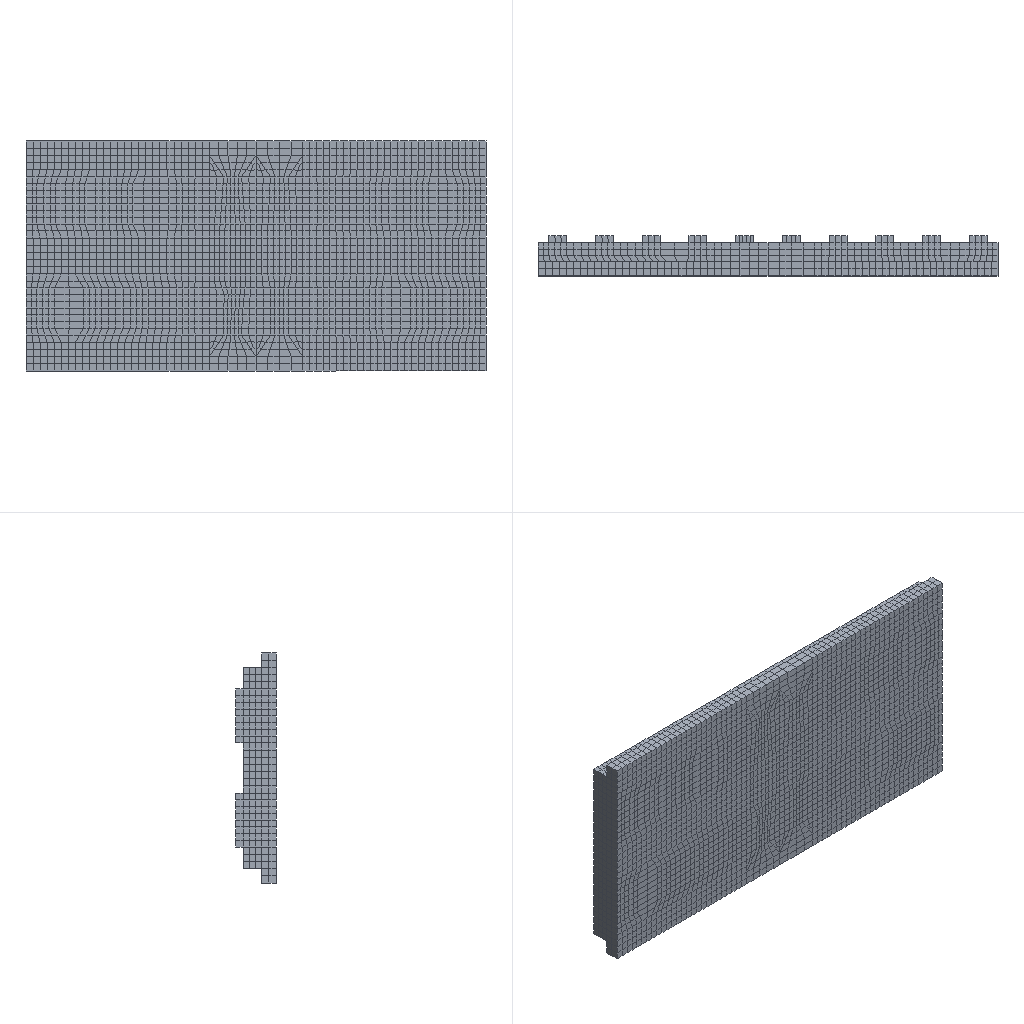Simulation study | abaqus
Set-up summary:
category,name,step,type,value,unit,region
solver,abaqus
solver,version,,,Abaqus/Explicit 2020
units,not stated in the deck,,not stated
analysis,deck,,transient,transient
load_step,Step-1,Step-1,transient,nlgeom=True
contact,interactions,,,general=0 pairs=0 ties=0
load_step,requested,,,1
mesh,nodes,,,15496
mesh,elements,,,12702
element_type,T3D2,,truss,1496
element_type,C3D8R,,solid,11134
element_type,COH3D8,,cohesive,72
load,load commands in deck,,count,1
bc,support commands in deck,,count,1
material,CONCRETE-COPY,,in results
material,CRACK,,in results
material,STEEL,,in results
check,setup vs results,,match,"per instance, exact: element labels, types and connectivity; labels of the nodes the elements use; coordinates not compared"
Abaqus input file, long lists of numbers shortened:
*Heading
** Job name: Job-2 Model name: Model-1
** Generated by: Abaqus/CAE 2020
*Preprint, echo=NO, model=NO, history=NO, contact=NO
**
** PARTS
**
*Part, name=concrete-final
*Node
      1,   4431.458,   309.396,        2750.
      2,   4431.458,   309.396,        3000.
** (14444 more lines like these left out)
*Element, type=C3D8R
 1,     4,   270,  2617,   277, 14216, 14215,  9263,  2648
 2,   270,   269,  2618,  2617, 14215, 14217,  9264,  9263
** (11132 more lines like these left out)
*Element, type=COH3D8
11135,   287,  2653,   270,     4, 14216, 14215,   270,     4
11136,  2653,  2654,   269,   270, 14215, 14217,   269,   270
** (70 more lines like these left out)
*Nset, nset=Set-17
     1,     2,     4,     5,     6,     7,     9,    10,    11,    12,    13,    14,    15,    16,    17,    18
    19,    20,    21,    22,    23,    24,    25,    26,    27,    28,    29,    30,    31,    32,    33,    34
** (851 more lines like these left out)
*Elset, elset=Set-17
   112,   113,   114,   115,   116,   117,   118,   119,   120,   121,   122,   123,   124,   125,   126,   127
   128,   129,   130,   131,   132,   133,   134,   135,   136,   137,   138,   139,   140,   141,   142,   143
** (660 more lines like these left out)
*Nset, nset=Set-22, generate
     1,  14286,      1
*Elset, elset=Set-22, generate
     1,  11134,      1
*Elset, elset=CohesiveSeam-2-Elements, generate
 11135,  11206,      1
*Nset, nset=CohesiveSeam-2-TopNodes
     1,     2,     3,     4,     6,     7,    11,    12,    13,    14,    15,    31,    32,    34,    49,    50
    51,    53,    54,    55,    56,    57,   269,   270,   275,   276,   281,   282,   283,   284,   309,   310
** (6 more lines like these left out)
*Nset, nset=CohesiveSeam-2-BottomNodes
    1,    2,    3,    4,    5,    6,    7,    8,   11,   12,   13,   14,   15,   16,   31,   32
   34,   35,   49,   50,   51,   52,   53,   54,   55,   56,   57,   58,  269,  270,  275,  276
** (6 more lines like these left out)
*Nset, nset=CohesiveSeam-2-MidNodes
   1,   2,   3,   4,   6,   7,  11,  12,  13,  14,  15,  31,  32,  34,  49,  50
  51,  53,  54,  55,  56,  57, 269, 270, 275, 276, 281, 282, 283, 284, 309, 310
** (2 more lines like these left out)
*Elset, elset=__PickedSurf72_S1, internal
 11135, 11136, 11137, 11138, 11139, 11140, 11141, 11142, 11143, 11153, 11154, 11155, 11156, 11157, 11158, 11159
 11160, 11161, 11189, 11190, 11191, 11192, 11193, 11194, 11195, 11196, 11197
*Elset, elset=__PickedSurf72_S2, internal
 11144, 11145, 11146, 11147, 11148, 11149, 11150, 11151, 11152, 11162, 11163, 11164, 11165, 11166, 11167, 11168
 11169, 11170, 11171, 11172, 11173, 11174, 11175, 11176, 11177, 11178, 11179, 11180, 11181, 11182, 11183, 11184
** (1 more lines like these left out)
*Surface, type=ELEMENT, name=_PickedSurf72, internal
__PickedSurf72_S1, S1
__PickedSurf72_S2, S2
*Elset, elset=_CohesiveSeam-2-TopSurf_S2, internal, generate
 11135,  11206,      1
*Surface, type=ELEMENT, name=CohesiveSeam-2-TopSurf
_CohesiveSeam-2-TopSurf_S2, S2
*Elset, elset=_CohesiveSeam-2-BottomSurf_S1, internal, generate
 11135,  11206,      1
*Surface, type=ELEMENT, name=CohesiveSeam-2-BottomSurf
_CohesiveSeam-2-BottomSurf_S1, S1
** Section: Section-1-SET-1
*Solid Section, elset=Set-22, material=CONCRETE-Copy
,
** Section: Section-coh
*Cohesive Section, elset=CohesiveSeam-2-Elements, controls=EC-1, material=crack, response=TRACTION SEPARATION, thickness=SPECIFIED
0.1,
*End Part
**
*Part, name="steel bar"
*Node
      1,       -1800.,        -350.,        2700.
      2,       -1400.,        -350.,        2700.
** (1048 more lines like these left out)
*Element, type=T3D2
   1,    1,  523
   2,  523,    2
** (1494 more lines like these left out)
*Nset, nset=SET-1, generate
    1,  1050,     1
*Elset, elset=SET-1, generate
    1,  1496,     1
*Nset, nset="'Set-300'", generate
    1,  1050,     1
*Nset, nset=Set-300
   1,  29,  37, 242, 266, 274, 350, 429
** Section: Section-2-SET-1
*Solid Section, elset=SET-1, material=STEEL
201.1,
*End Part
**
**
** ASSEMBLY
**
*Assembly, name=Assembly
**
*Instance, name="steel bar-1", part="steel bar"
*End Instance
**
*Instance, name=concrete-final-1, part=concrete-final
      -1850.,  -709.396,  4731.457
      -1850.,  -709.396,  4731.457,       -1850., -708.396,  4731.457, 90.
*End Instance
**
*Node
      1,        1025.,         -40.,        2125.
      2,        1675.,         -40.,        2125.
** (5 more lines like these left out)
*Nset, nset=M_SET-1
 1,
*Nset, nset=M_SET-2
 2,
*Nset, nset=M_SET-3
 4,
*Nset, nset=M_SET-4
 3,
*Nset, nset=M_SET-12
 6,
*Nset, nset=M_SET-13
 7,
*Nset, nset=M_SET-16
 5,
*Nset, nset=SET-10, generate
 1,  4,  1
*Nset, nset=SET-11
 5,
*Nset, nset=SET-14
 7,
*Nset, nset=SET-15
 6,
*Nset, nset=SET-17
 5,
*Nset, nset=Set-41, instance=concrete-final-1
   19,   20,   21,   22,   37,   38,   39,   40,   61,   62,   63,   64,   80,   81,   82,   83
   84,   86,   87,  112,  113,  114,  115,  116,  117,  141,  142,  143,  153,  154,  155,  156
** (22 more lines like these left out)
*Elset, elset=Set-41, instance=concrete-final-1
   346,   347,   348,   349,   350,   351,   352,   353,   354,   604,   605,   606,   607,   608,   609,   610
   611,   612,   934,   935,   936,   937,   938,   939,   940,   941,   942,  1263,  1264,  1265,  1266,  1267
** (18 more lines like these left out)
*Nset, nset=Set-42, generate
 1,  4,  1
*Nset, nset=WIRE-1-SET-2, instance="steel bar-1", generate
    1,  1050,     1
*Nset, nset=m_Set-35
 1,
*Nset, nset=m_Set-36
 2,
*Nset, nset=m_Set-37
 3,
*Nset, nset=m_Set-38
 4,
*Elset, elset=m_Set-39, instance="steel bar-1", generate
    1,  1496,     1
*Elset, elset=m_Set-42, instance="steel bar-1", generate
    1,  1496,     1
*Nset, nset=s_Set-39, instance=concrete-final-1
     1,     2,     4,     5,     6,     7,     9,    10,    11,    12,    13,    14,    15,    16,    17,    18
    19,    20,    21,    22,    23,    24,    25,    26,    27,    28,    29,    30,    31,    32,    33,    34
** (851 more lines like these left out)
*Elset, elset=s_Set-39, instance=concrete-final-1
   112,   113,   114,   115,   116,   117,   118,   119,   120,   121,   122,   123,   124,   125,   126,   127
   128,   129,   130,   131,   132,   133,   134,   135,   136,   137,   138,   139,   140,   141,   142,   143
** (660 more lines like these left out)
*Nset, nset=s_Set-42, instance=concrete-final-1, generate
     1,  14286,      1
*Elset, elset=s_Set-42, instance=concrete-final-1, generate
     1,  11134,      1
*Elset, elset=_s_Surf-9_S5, internal, instance=concrete-final-1, generate
 8271,  8310,     1
*Surface, type=ELEMENT, name=s_Surf-9
_s_Surf-9_S5, S5
*Elset, elset=_s_Surf-10_S5, internal, instance=concrete-final-1, generate
 5079,  5110,     1
*Surface, type=ELEMENT, name=s_Surf-10
_s_Surf-10_S5, S5
*Elset, elset=_s_Surf-11_S5, internal, instance=concrete-final-1, generate
 5207,  5238,     1
*Surface, type=ELEMENT, name=s_Surf-11
_s_Surf-11_S5, S5
*Elset, elset=_s_Surf-12_S5, internal, instance=concrete-final-1, generate
 6695,  6734,     1
*Surface, type=ELEMENT, name=s_Surf-12
_s_Surf-12_S5, S5
** Constraint: CONSTRAINT-1
*Coupling, constraint name=CONSTRAINT-1, ref node=m_Set-35, surface=s_Surf-9
*Kinematic
** Constraint: CONSTRAINT-2
*Coupling, constraint name=CONSTRAINT-2, ref node=m_Set-36, surface=s_Surf-10
*Kinematic
** Constraint: CONSTRAINT-3
*Coupling, constraint name=CONSTRAINT-3, ref node=m_Set-37, surface=s_Surf-11
*Kinematic
** Constraint: CONSTRAINT-4
*Coupling, constraint name=CONSTRAINT-4, ref node=m_Set-38, surface=s_Surf-12
*Kinematic
** Constraint: Constraint-6
*Embedded Element, host elset=s_Set-42
m_Set-42
*End Assembly
**
** ELEMENT CONTROLS
**
*Section Controls, name=EC-1, ELEMENT DELETION=YES
1., 1., 1.
*Amplitude, name=AMP-1
             0.,              1.,            0.05,              1.
*Amplitude, name=AMP-2
             0.,             0.2,           0.025,            1.76,            0.05,             0.2
*Amplitude, name=AMP-3
             0.,              1.,            0.05,              1.
*Amplitude, name=AMP-4
             0.,             0.2,            0.05,            1.75,             0.1,             0.2
*Amplitude, name=AMP-5
             0.,              1.,             0.1,              1.
**
** MATERIALS
**
*Material, name=CONCRETE-Copy
*Density
 2.35e-09,
*Elastic
36000., 0.2
*Material, name=STEEL
*Density
 7.85e-09,
*Elastic
200000., 0.3
*Plastic
400.,0.
*Material, name=crack
*Damage Initiation, criterion=MAXS
 1.5, 1.5, 1.5
*Damage Evolution, type=DISPLACEMENT
 0.001,
*Density
 2.35e-09,
*Elastic, type=TRACTION
36000.,36000.,36000.
**
** INTERACTION PROPERTIES
**
*Surface Interaction, name=XFEM
*Friction
 0.01,
*Surface Behavior, pressure-overclosure=HARD
** ----------------------------------------------------------------
**
** STEP: Step-1
**
*Step, name=Step-1, nlgeom=YES
*Dynamic, Explicit
, 0.1
*Bulk Viscosity
0.06, 1.2
** Mass Scaling: Semi-Automatic
**               Whole Model
*Fixed Mass Scaling, factor=50.
**
** BOUNDARY CONDITIONS
**
** Name: BC-1 Type: 对称/反对称/完全固定
*Boundary
Set-41, ENCASTRE
**
** LOADS
**
** Name: Load-1   Type: Concentrated force
*Cload, amplitude=AMP-4
Set-42, 2, -85000.
**
** OUTPUT REQUESTS
**
*Restart, write, number interval=1, time marks=NO
**
** FIELD OUTPUT: F-Output-1
**
*Output, field, number interval=50
*Node Output
A, RF, RT, U, V
*Element Output, directions=YES
E, EVF, LE, MISES, MISESMAX, PE, PEEQ, PEEQVAVG, PEVAVG, S, SDEG, SSAVG, STATUS, SVAVG
*Contact Output
CDISP, CSDMG, CSTRESS
**
** HISTORY OUTPUT: H-Output-1
**
*Output, history, variable=PRESELECT, frequency=1
*End Step
Results summary:
result,step,Step-1,completed,increments=37861 time=0.1/0.1
result,analysis,,,transient
result,last_loadstep,,,1
result,analysis steps,,count,1
result,primary field,,,U
result,reaction total,,FX,1664.502,model units
result,reaction total,,FY,1048001.884,model units
result,reaction total,,FZ,2070.716,model units